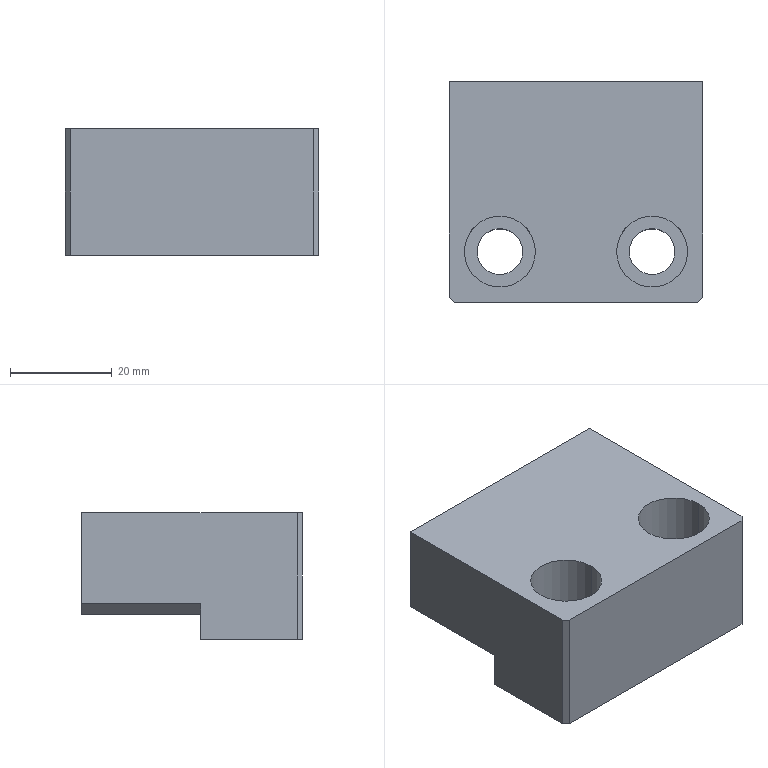Part | STEP file | J454-EBZ05-28-00-Part-1 | 1 solid | 36 faces | box 50 x 43.5 x 25 mm | volume 41584 mm3 | cylinder 16 | plane 16 | cone 4 | commonest cylinder face diameters 6.9 x4 8 x4 9 x4 14 x4
STEP:
#1=CARTESIAN_POINT('',(-15.,13.427,5.));
#2=VERTEX_POINT('',#1);
#3=CARTESIAN_POINT('',(-15.,15.5,8.45));
#4=VERTEX_POINT('',#3);
#5=CARTESIAN_POINT('',(-15.,15.5,8.45));
#6=DIRECTION('',(0.,0.515,0.8572));
#7=VECTOR('',#6,1000.);
#8=LINE('',#5,#7);
#9=EDGE_CURVE('',#2,#4,#8,.T.);
#10=ORIENTED_EDGE('',*,*,#9,.F.);
#11=CARTESIAN_POINT('',(-15.,15.5,1.55));
#12=VERTEX_POINT('',#11);
#13=CARTESIAN_POINT('',(-15.,15.5,1.55));
#14=DIRECTION('',(0.,0.515,-0.8572));
#15=VECTOR('',#14,1000.);
#16=LINE('',#13,#15);
#17=EDGE_CURVE('',#2,#12,#16,.T.);
#18=ORIENTED_EDGE('',*,*,#17,.T.);
#19=CARTESIAN_POINT('',(-15.,15.5,5.));
#20=DIRECTION('',(0.,1.,0.));
#21=DIRECTION('',(0.,0.,1.));
#22=AXIS2_PLACEMENT_3D('',#19,#20,#21);
#23=CIRCLE('',#22,3.45);
#24=EDGE_CURVE('',#12,#4,#23,.T.);
#25=ORIENTED_EDGE('',*,*,#24,.T.);
#26=EDGE_LOOP('',(#10,#18,#25));
#27=FACE_OUTER_BOUND('',#26,.T.);
#28=CARTESIAN_POINT('',(-15.,15.5,5.));
#29=DIRECTION('',(0.,1.,0.));
#30=DIRECTION('',(0.,0.,1.));
#31=AXIS2_PLACEMENT_3D('',#28,#29,#30);
#32=CONICAL_SURFACE('',#31,3.45,1.03);
#33=ADVANCED_FACE('',(#27),#32,.F.);
#34=ORIENTED_EDGE('',*,*,#24,.F.);
#35=CARTESIAN_POINT('',(-15.,17.5,1.55));
#36=VERTEX_POINT('',#35);
#37=CARTESIAN_POINT('',(-15.,33.5,1.55));
#38=DIRECTION('',(0.,1.,0.));
#39=VECTOR('',#38,1000.);
#40=LINE('',#37,#39);
#41=EDGE_CURVE('',#12,#36,#40,.T.);
#42=ORIENTED_EDGE('',*,*,#41,.T.);
#43=CARTESIAN_POINT('',(-15.,17.5,8.45));
#44=VERTEX_POINT('',#43);
#45=CARTESIAN_POINT('',(-15.,17.5,5.));
#46=DIRECTION('',(0.,1.,0.));
#47=DIRECTION('',(0.,0.,1.));
#48=AXIS2_PLACEMENT_3D('',#45,#46,#47);
#49=CIRCLE('',#48,3.45);
#50=EDGE_CURVE('',#36,#44,#49,.T.);
#51=ORIENTED_EDGE('',*,*,#50,.T.);
#52=CARTESIAN_POINT('',(-15.,33.5,8.45));
#53=DIRECTION('',(0.,1.,0.));
#54=VECTOR('',#53,1000.);
#55=LINE('',#52,#54);
#56=EDGE_CURVE('',#4,#44,#55,.T.);
#57=ORIENTED_EDGE('',*,*,#56,.F.);
#58=EDGE_LOOP('',(#34,#42,#51,#57));
#59=FACE_OUTER_BOUND('',#58,.T.);
#60=CARTESIAN_POINT('',(-15.,33.5,5.));
#61=DIRECTION('',(0.,1.,0.));
#62=DIRECTION('',(0.,0.,1.));
#63=AXIS2_PLACEMENT_3D('',#60,#61,#62);
#64=CYLINDRICAL_SURFACE('',#63,3.45);
#65=ADVANCED_FACE('',(#59),#64,.F.);
#66=CARTESIAN_POINT('',(-15.,17.5,1.));
#67=VERTEX_POINT('',#66);
#68=CARTESIAN_POINT('',(-15.,17.5,9.));
#69=VERTEX_POINT('',#68);
#70=CARTESIAN_POINT('',(-15.,17.5,5.));
#71=DIRECTION('',(0.,1.,0.));
#72=DIRECTION('',(0.,0.,1.));
#73=AXIS2_PLACEMENT_3D('',#70,#71,#72);
#74=CIRCLE('',#73,4.);
#75=EDGE_CURVE('',#67,#69,#74,.T.);
#76=ORIENTED_EDGE('',*,*,#75,.F.);
#77=CARTESIAN_POINT('',(-15.,33.5,1.));
#78=VERTEX_POINT('',#77);
#79=CARTESIAN_POINT('',(-15.,33.5,1.));
#80=DIRECTION('',(0.,1.,0.));
#81=VECTOR('',#80,1000.);
#82=LINE('',#79,#81);
#83=EDGE_CURVE('',#67,#78,#82,.T.);
#84=ORIENTED_EDGE('',*,*,#83,.T.);
#85=CARTESIAN_POINT('',(-15.,33.5,9.));
#86=VERTEX_POINT('',#85);
#87=CARTESIAN_POINT('',(-15.,33.5,5.));
#88=DIRECTION('',(0.,1.,0.));
#89=DIRECTION('',(0.,0.,1.));
#90=AXIS2_PLACEMENT_3D('',#87,#88,#89);
#91=CIRCLE('',#90,4.);
#92=EDGE_CURVE('',#78,#86,#91,.T.);
#93=ORIENTED_EDGE('',*,*,#92,.T.);
#94=CARTESIAN_POINT('',(-15.,33.5,9.));
#95=DIRECTION('',(0.,1.,0.));
#96=VECTOR('',#95,1000.);
#97=LINE('',#94,#96);
#98=EDGE_CURVE('',#69,#86,#97,.T.);
#99=ORIENTED_EDGE('',*,*,#98,.F.);
#100=EDGE_LOOP('',(#76,#84,#93,#99));
#101=FACE_OUTER_BOUND('',#100,.T.);
#102=CARTESIAN_POINT('',(-15.,33.5,5.));
#103=DIRECTION('',(0.,1.,0.));
#104=DIRECTION('',(0.,0.,1.));
#105=AXIS2_PLACEMENT_3D('',#102,#103,#104);
#106=CYLINDRICAL_SURFACE('',#105,4.);
#107=ADVANCED_FACE('',(#101),#106,.F.);
#108=CARTESIAN_POINT('',(15.,13.427,5.));
#109=VERTEX_POINT('',#108);
#110=CARTESIAN_POINT('',(15.,15.5,8.45));
#111=VERTEX_POINT('',#110);
#112=CARTESIAN_POINT('',(15.,15.5,8.45));
#113=DIRECTION('',(0.,0.515,0.8572));
#114=VECTOR('',#113,1000.);
#115=LINE('',#112,#114);
#116=EDGE_CURVE('',#109,#111,#115,.T.);
#117=ORIENTED_EDGE('',*,*,#116,.F.);
#118=CARTESIAN_POINT('',(15.,15.5,1.55));
#119=VERTEX_POINT('',#118);
#120=CARTESIAN_POINT('',(15.,15.5,1.55));
#121=DIRECTION('',(0.,0.515,-0.8572));
#122=VECTOR('',#121,1000.);
#123=LINE('',#120,#122);
#124=EDGE_CURVE('',#109,#119,#123,.T.);
#125=ORIENTED_EDGE('',*,*,#124,.T.);
#126=CARTESIAN_POINT('',(15.,15.5,5.));
#127=DIRECTION('',(0.,1.,0.));
#128=DIRECTION('',(0.,0.,1.));
#129=AXIS2_PLACEMENT_3D('',#126,#127,#128);
#130=CIRCLE('',#129,3.45);
#131=EDGE_CURVE('',#119,#111,#130,.T.);
#132=ORIENTED_EDGE('',*,*,#131,.T.);
#133=EDGE_LOOP('',(#117,#125,#132));
#134=FACE_OUTER_BOUND('',#133,.T.);
#135=CARTESIAN_POINT('',(15.,15.5,5.));
#136=DIRECTION('',(0.,1.,0.));
#137=DIRECTION('',(0.,0.,1.));
#138=AXIS2_PLACEMENT_3D('',#135,#136,#137);
#139=CONICAL_SURFACE('',#138,3.45,1.03);
#140=ADVANCED_FACE('',(#134),#139,.F.);
#141=ORIENTED_EDGE('',*,*,#131,.F.);
#142=CARTESIAN_POINT('',(15.,17.5,1.55));
#143=VERTEX_POINT('',#142);
#144=CARTESIAN_POINT('',(15.,33.5,1.55));
#145=DIRECTION('',(0.,1.,0.));
#146=VECTOR('',#145,1000.);
#147=LINE('',#144,#146);
#148=EDGE_CURVE('',#119,#143,#147,.T.);
#149=ORIENTED_EDGE('',*,*,#148,.T.);
#150=CARTESIAN_POINT('',(15.,17.5,8.45));
#151=VERTEX_POINT('',#150);
#152=CARTESIAN_POINT('',(15.,17.5,5.));
#153=DIRECTION('',(0.,1.,0.));
#154=DIRECTION('',(0.,0.,1.));
#155=AXIS2_PLACEMENT_3D('',#152,#153,#154);
#156=CIRCLE('',#155,3.45);
#157=EDGE_CURVE('',#143,#151,#156,.T.);
#158=ORIENTED_EDGE('',*,*,#157,.T.);
#159=CARTESIAN_POINT('',(15.,33.5,8.45));
#160=DIRECTION('',(0.,1.,0.));
#161=VECTOR('',#160,1000.);
#162=LINE('',#159,#161);
#163=EDGE_CURVE('',#111,#151,#162,.T.);
#164=ORIENTED_EDGE('',*,*,#163,.F.);
#165=EDGE_LOOP('',(#141,#149,#158,#164));
#166=FACE_OUTER_BOUND('',#165,.T.);
#167=CARTESIAN_POINT('',(15.,33.5,5.));
#168=DIRECTION('',(0.,1.,0.));
#169=DIRECTION('',(0.,0.,1.));
#170=AXIS2_PLACEMENT_3D('',#167,#168,#169);
#171=CYLINDRICAL_SURFACE('',#170,3.45);
#172=ADVANCED_FACE('',(#166),#171,.F.);
#173=CARTESIAN_POINT('',(15.,17.5,1.));
#174=VERTEX_POINT('',#173);
#175=CARTESIAN_POINT('',(15.,17.5,9.));
#176=VERTEX_POINT('',#175);
#177=CARTESIAN_POINT('',(15.,17.5,5.));
#178=DIRECTION('',(0.,1.,0.));
#179=DIRECTION('',(0.,0.,1.));
#180=AXIS2_PLACEMENT_3D('',#177,#178,#179);
#181=CIRCLE('',#180,4.);
#182=EDGE_CURVE('',#174,#176,#181,.T.);
#183=ORIENTED_EDGE('',*,*,#182,.F.);
#184=CARTESIAN_POINT('',(15.,33.5,1.));
#185=VERTEX_POINT('',#184);
#186=CARTESIAN_POINT('',(15.,33.5,1.));
#187=DIRECTION('',(0.,1.,0.));
#188=VECTOR('',#187,1000.);
#189=LINE('',#186,#188);
#190=EDGE_CURVE('',#174,#185,#189,.T.);
#191=ORIENTED_EDGE('',*,*,#190,.T.);
#192=CARTESIAN_POINT('',(15.,33.5,9.));
#193=VERTEX_POINT('',#192);
#194=CARTESIAN_POINT('',(15.,33.5,5.));
#195=DIRECTION('',(0.,1.,0.));
#196=DIRECTION('',(0.,0.,1.));
#197=AXIS2_PLACEMENT_3D('',#194,#195,#196);
#198=CIRCLE('',#197,4.);
#199=EDGE_CURVE('',#185,#193,#198,.T.);
#200=ORIENTED_EDGE('',*,*,#199,.T.);
#201=CARTESIAN_POINT('',(15.,33.5,9.));
#202=DIRECTION('',(0.,1.,0.));
#203=VECTOR('',#202,1000.);
#204=LINE('',#201,#203);
#205=EDGE_CURVE('',#176,#193,#204,.T.);
#206=ORIENTED_EDGE('',*,*,#205,.F.);
#207=EDGE_LOOP('',(#183,#191,#200,#206));
#208=FACE_OUTER_BOUND('',#207,.T.);
#209=CARTESIAN_POINT('',(15.,33.5,5.));
#210=DIRECTION('',(0.,1.,0.));
#211=DIRECTION('',(0.,0.,1.));
#212=AXIS2_PLACEMENT_3D('',#209,#210,#211);
#213=CYLINDRICAL_SURFACE('',#212,4.);
#214=ADVANCED_FACE('',(#208),#213,.F.);
#215=CARTESIAN_POINT('',(19.5,0.,-10.));
#216=VERTEX_POINT('',#215);
#217=CARTESIAN_POINT('',(10.5,0.,-10.));
#218=VERTEX_POINT('',#217);
#219=CARTESIAN_POINT('',(15.,0.,-10.));
#220=DIRECTION('',(0.,0.,1.));
#221=DIRECTION('',(-1.,0.,0.));
#222=AXIS2_PLACEMENT_3D('',#219,#220,#221);
#223=CIRCLE('',#222,4.5);
#224=EDGE_CURVE('',#216,#218,#223,.T.);
#225=ORIENTED_EDGE('',*,*,#224,.F.);
#226=CARTESIAN_POINT('',(19.5,0.,5.));
#227=VERTEX_POINT('',#226);
#228=CARTESIAN_POINT('',(19.5,0.,15.));
#229=DIRECTION('',(0.,0.,1.));
#230=VECTOR('',#229,1000.);
#231=LINE('',#228,#230);
#232=EDGE_CURVE('',#216,#227,#231,.T.);
#233=ORIENTED_EDGE('',*,*,#232,.T.);
#234=CARTESIAN_POINT('',(10.5,0.,5.));
#235=VERTEX_POINT('',#234);
#236=CARTESIAN_POINT('',(15.,0.,5.));
#237=DIRECTION('',(0.,0.,1.));
#238=DIRECTION('',(-1.,0.,0.));
#239=AXIS2_PLACEMENT_3D('',#236,#237,#238);
#240=CIRCLE('',#239,4.5);
#241=EDGE_CURVE('',#227,#235,#240,.T.);
#242=ORIENTED_EDGE('',*,*,#241,.T.);
#243=CARTESIAN_POINT('',(10.5,0.,15.));
#244=DIRECTION('',(0.,0.,1.));
#245=VECTOR('',#244,1000.);
#246=LINE('',#243,#245);
#247=EDGE_CURVE('',#218,#235,#246,.T.);
#248=ORIENTED_EDGE('',*,*,#247,.F.);
#249=EDGE_LOOP('',(#225,#233,#242,#248));
#250=FACE_OUTER_BOUND('',#249,.T.);
#251=CARTESIAN_POINT('',(15.,0.,15.));
#252=DIRECTION('',(0.,0.,1.));
#253=DIRECTION('',(-1.,0.,0.));
#254=AXIS2_PLACEMENT_3D('',#251,#252,#253);
#255=CYLINDRICAL_SURFACE('',#254,4.5);
#256=ADVANCED_FACE('',(#250),#255,.F.);
#257=CARTESIAN_POINT('',(22.,0.,5.));
#258=VERTEX_POINT('',#257);
#259=CARTESIAN_POINT('',(8.,0.,5.));
#260=VERTEX_POINT('',#259);
#261=CARTESIAN_POINT('',(15.,0.,5.));
#262=DIRECTION('',(0.,0.,1.));
#263=DIRECTION('',(-1.,0.,0.));
#264=AXIS2_PLACEMENT_3D('',#261,#262,#263);
#265=CIRCLE('',#264,7.);
#266=EDGE_CURVE('',#258,#260,#265,.T.);
#267=ORIENTED_EDGE('',*,*,#266,.F.);
#268=CARTESIAN_POINT('',(22.,0.,15.));
#269=VERTEX_POINT('',#268);
#270=CARTESIAN_POINT('',(22.,0.,15.));
#271=DIRECTION('',(0.,0.,1.));
#272=VECTOR('',#271,1000.);
#273=LINE('',#270,#272);
#274=EDGE_CURVE('',#258,#269,#273,.T.);
#275=ORIENTED_EDGE('',*,*,#274,.T.);
#276=CARTESIAN_POINT('',(8.,0.,15.));
#277=VERTEX_POINT('',#276);
#278=CARTESIAN_POINT('',(15.,0.,15.));
#279=DIRECTION('',(0.,0.,1.));
#280=DIRECTION('',(-1.,0.,0.));
#281=AXIS2_PLACEMENT_3D('',#278,#279,#280);
#282=CIRCLE('',#281,7.);
#283=EDGE_CURVE('',#269,#277,#282,.T.);
#284=ORIENTED_EDGE('',*,*,#283,.T.);
#285=CARTESIAN_POINT('',(8.,0.,15.));
#286=DIRECTION('',(0.,0.,1.));
#287=VECTOR('',#286,1000.);
#288=LINE('',#285,#287);
#289=EDGE_CURVE('',#260,#277,#288,.T.);
#290=ORIENTED_EDGE('',*,*,#289,.F.);
#291=EDGE_LOOP('',(#267,#275,#284,#290));
#292=FACE_OUTER_BOUND('',#291,.T.);
#293=CARTESIAN_POINT('',(15.,0.,15.));
#294=DIRECTION('',(0.,0.,1.));
#295=DIRECTION('',(-1.,0.,0.));
#296=AXIS2_PLACEMENT_3D('',#293,#294,#295);
#297=CYLINDRICAL_SURFACE('',#296,7.);
#298=ADVANCED_FACE('',(#292),#297,.F.);
#299=CARTESIAN_POINT('',(-10.5,0.,-10.));
#300=VERTEX_POINT('',#299);
#301=CARTESIAN_POINT('',(-19.5,0.,-10.));
#302=VERTEX_POINT('',#301);
#303=CARTESIAN_POINT('',(-15.,0.,-10.));
#304=DIRECTION('',(0.,0.,1.));
#305=DIRECTION('',(-1.,0.,0.));
#306=AXIS2_PLACEMENT_3D('',#303,#304,#305);
#307=CIRCLE('',#306,4.5);
#308=EDGE_CURVE('',#300,#302,#307,.T.);
#309=ORIENTED_EDGE('',*,*,#308,.F.);
#310=CARTESIAN_POINT('',(-10.5,0.,5.));
#311=VERTEX_POINT('',#310);
#312=CARTESIAN_POINT('',(-10.5,0.,15.));
#313=DIRECTION('',(0.,0.,1.));
#314=VECTOR('',#313,1000.);
#315=LINE('',#312,#314);
#316=EDGE_CURVE('',#300,#311,#315,.T.);
#317=ORIENTED_EDGE('',*,*,#316,.T.);
#318=CARTESIAN_POINT('',(-19.5,0.,5.));
#319=VERTEX_POINT('',#318);
#320=CARTESIAN_POINT('',(-15.,0.,5.));
#321=DIRECTION('',(0.,0.,1.));
#322=DIRECTION('',(-1.,0.,0.));
#323=AXIS2_PLACEMENT_3D('',#320,#321,#322);
#324=CIRCLE('',#323,4.5);
#325=EDGE_CURVE('',#311,#319,#324,.T.);
#326=ORIENTED_EDGE('',*,*,#325,.T.);
#327=CARTESIAN_POINT('',(-19.5,0.,15.));
#328=DIRECTION('',(0.,0.,1.));
#329=VECTOR('',#328,1000.);
#330=LINE('',#327,#329);
#331=EDGE_CURVE('',#302,#319,#330,.T.);
#332=ORIENTED_EDGE('',*,*,#331,.F.);
#333=EDGE_LOOP('',(#309,#317,#326,#332));
#334=FACE_OUTER_BOUND('',#333,.T.);
#335=CARTESIAN_POINT('',(-15.,0.,15.));
#336=DIRECTION('',(0.,0.,1.));
#337=DIRECTION('',(-1.,0.,0.));
#338=AXIS2_PLACEMENT_3D('',#335,#336,#337);
#339=CYLINDRICAL_SURFACE('',#338,4.5);
#340=ADVANCED_FACE('',(#334),#339,.F.);
#341=CARTESIAN_POINT('',(-8.,0.,5.));
#342=VERTEX_POINT('',#341);
#343=CARTESIAN_POINT('',(-22.,0.,5.));
#344=VERTEX_POINT('',#343);
#345=CARTESIAN_POINT('',(-15.,0.,5.));
#346=DIRECTION('',(0.,0.,1.));
#347=DIRECTION('',(-1.,0.,0.));
#348=AXIS2_PLACEMENT_3D('',#345,#346,#347);
#349=CIRCLE('',#348,7.);
#350=EDGE_CURVE('',#342,#344,#349,.T.);
#351=ORIENTED_EDGE('',*,*,#350,.F.);
#352=CARTESIAN_POINT('',(-8.,0.,15.));
#353=VERTEX_POINT('',#352);
#354=CARTESIAN_POINT('',(-8.,0.,15.));
#355=DIRECTION('',(0.,0.,1.));
#356=VECTOR('',#355,1000.);
#357=LINE('',#354,#356);
#358=EDGE_CURVE('',#342,#353,#357,.T.);
#359=ORIENTED_EDGE('',*,*,#358,.T.);
#360=CARTESIAN_POINT('',(-22.,0.,15.));
#361=VERTEX_POINT('',#360);
#362=CARTESIAN_POINT('',(-15.,0.,15.));
#363=DIRECTION('',(0.,0.,1.));
#364=DIRECTION('',(-1.,0.,0.));
#365=AXIS2_PLACEMENT_3D('',#362,#363,#364);
#366=CIRCLE('',#365,7.);
#367=EDGE_CURVE('',#353,#361,#366,.T.);
#368=ORIENTED_EDGE('',*,*,#367,.T.);
#369=CARTESIAN_POINT('',(-22.,0.,15.));
#370=DIRECTION('',(0.,0.,1.));
#371=VECTOR('',#370,1000.);
#372=LINE('',#369,#371);
#373=EDGE_CURVE('',#344,#361,#372,.T.);
#374=ORIENTED_EDGE('',*,*,#373,.F.);
#375=EDGE_LOOP('',(#351,#359,#368,#374));
#376=FACE_OUTER_BOUND('',#375,.T.);
#377=CARTESIAN_POINT('',(-15.,0.,15.));
#378=DIRECTION('',(0.,0.,1.));
#379=DIRECTION('',(-1.,0.,0.));
#380=AXIS2_PLACEMENT_3D('',#377,#378,#379);
#381=CYLINDRICAL_SURFACE('',#380,7.);
#382=ADVANCED_FACE('',(#376),#381,.F.);
#383=CARTESIAN_POINT('',(25.,10.,-10.));
#384=VERTEX_POINT('',#383);
#385=CARTESIAN_POINT('',(25.,10.,-3.));
#386=VERTEX_POINT('',#385);
#387=CARTESIAN_POINT('',(25.,10.,-10.));
#388=DIRECTION('',(0.,0.,1.));
#389=VECTOR('',#388,1000.);
#390=LINE('',#387,#389);
#391=EDGE_CURVE('',#384,#386,#390,.T.);
#392=ORIENTED_EDGE('',*,*,#391,.T.);
#393=CARTESIAN_POINT('',(25.,33.5,-3.));
#394=VERTEX_POINT('',#393);
#395=CARTESIAN_POINT('',(25.,21.905,-3.));
#396=DIRECTION('',(0.,1.,0.));
#397=VECTOR('',#396,1000.);
#398=LINE('',#395,#397);
#399=EDGE_CURVE('',#386,#394,#398,.T.);
#400=ORIENTED_EDGE('',*,*,#399,.T.);
#401=CARTESIAN_POINT('',(25.,33.5,15.));
#402=VERTEX_POINT('',#401);
#403=CARTESIAN_POINT('',(25.,33.5,-20.405));
#404=DIRECTION('',(0.,0.,-1.));
#405=VECTOR('',#404,1000.);
#406=LINE('',#403,#405);
#407=EDGE_CURVE('',#402,#394,#406,.T.);
#408=ORIENTED_EDGE('',*,*,#407,.F.);
#409=CARTESIAN_POINT('',(25.,-9.,15.));
#410=VERTEX_POINT('',#409);
#411=CARTESIAN_POINT('',(25.,-9.,15.));
#412=DIRECTION('',(0.,1.,0.));
#413=VECTOR('',#412,1000.);
#414=LINE('',#411,#413);
#415=EDGE_CURVE('',#410,#402,#414,.T.);
#416=ORIENTED_EDGE('',*,*,#415,.F.);
#417=CARTESIAN_POINT('',(25.,-9.,-10.));
#418=VERTEX_POINT('',#417);
#419=CARTESIAN_POINT('',(25.,-9.,13.));
#420=DIRECTION('',(0.,0.,-1.));
#421=VECTOR('',#420,1000.);
#422=LINE('',#419,#421);
#423=EDGE_CURVE('',#410,#418,#422,.T.);
#424=ORIENTED_EDGE('',*,*,#423,.T.);
#425=CARTESIAN_POINT('',(25.,9.,-10.));
#426=DIRECTION('',(0.,-1.,0.));
#427=VECTOR('',#426,1000.);
#428=LINE('',#425,#427);
#429=EDGE_CURVE('',#384,#418,#428,.T.);
#430=ORIENTED_EDGE('',*,*,#429,.F.);
#431=EDGE_LOOP('',(#392,#400,#408,#416,#424,#430));
#432=FACE_OUTER_BOUND('',#431,.T.);
#433=CARTESIAN_POINT('',(25.,21.905,-20.405));
#434=DIRECTION('',(-1.,0.,0.));
#435=DIRECTION('',(0.,-1.,0.));
#436=AXIS2_PLACEMENT_3D('',#433,#434,#435);
#437=PLANE('',#436);
#438=ADVANCED_FACE('',(#432),#437,.F.);
#439=CARTESIAN_POINT('',(15.,0.,-10.));
#440=DIRECTION('',(0.,0.,1.));
#441=DIRECTION('',(-1.,0.,0.));
#442=AXIS2_PLACEMENT_3D('',#439,#440,#441);
#443=CIRCLE('',#442,4.5);
#444=EDGE_CURVE('',#218,#216,#443,.T.);
#445=ORIENTED_EDGE('',*,*,#444,.T.);
#446=ORIENTED_EDGE('',*,*,#224,.T.);
#447=EDGE_LOOP('',(#445,#446));
#448=FACE_BOUND('',#447,.T.);
#449=CARTESIAN_POINT('',(-15.,0.,-10.));
#450=DIRECTION('',(0.,0.,1.));
#451=DIRECTION('',(-1.,0.,0.));
#452=AXIS2_PLACEMENT_3D('',#449,#450,#451);
#453=CIRCLE('',#452,4.5);
#454=EDGE_CURVE('',#302,#300,#453,.T.);
#455=ORIENTED_EDGE('',*,*,#454,.T.);
#456=ORIENTED_EDGE('',*,*,#308,.T.);
#457=EDGE_LOOP('',(#455,#456));
#458=FACE_BOUND('',#457,.T.);
#459=CARTESIAN_POINT('',(-25.,10.,-10.));
#460=VERTEX_POINT('',#459);
#461=CARTESIAN_POINT('',(-25.,-9.,-10.));
#462=VERTEX_POINT('',#461);
#463=CARTESIAN_POINT('',(-25.,9.,-10.));
#464=DIRECTION('',(0.,-1.,0.));
#465=VECTOR('',#464,1000.);
#466=LINE('',#463,#465);
#467=EDGE_CURVE('',#460,#462,#466,.T.);
#468=ORIENTED_EDGE('',*,*,#467,.F.);
#469=CARTESIAN_POINT('',(0.,10.,-10.));
#470=DIRECTION('',(1.,0.,0.));
#471=VECTOR('',#470,1000.);
#472=LINE('',#469,#471);
#473=EDGE_CURVE('',#460,#384,#472,.T.);
#474=ORIENTED_EDGE('',*,*,#473,.T.);
#475=ORIENTED_EDGE('',*,*,#429,.T.);
#476=CARTESIAN_POINT('',(24.,-10.,-10.));
#477=VERTEX_POINT('',#476);
#478=CARTESIAN_POINT('',(25.,-9.,-10.));
#479=DIRECTION('',(-0.7071,-0.7071,0.));
#480=VECTOR('',#479,1000.);
#481=LINE('',#478,#480);
#482=EDGE_CURVE('',#418,#477,#481,.T.);
#483=ORIENTED_EDGE('',*,*,#482,.T.);
#484=CARTESIAN_POINT('',(-24.,-10.,-10.));
#485=VERTEX_POINT('',#484);
#486=CARTESIAN_POINT('',(24.,-10.,-10.));
#487=DIRECTION('',(-1.,0.,0.));
#488=VECTOR('',#487,1000.);
#489=LINE('',#486,#488);
#490=EDGE_CURVE('',#477,#485,#489,.T.);
#491=ORIENTED_EDGE('',*,*,#490,.T.);
#492=CARTESIAN_POINT('',(-24.,-10.,-10.));
#493=DIRECTION('',(-0.7071,0.7071,0.));
#494=VECTOR('',#493,1000.);
#495=LINE('',#492,#494);
#496=EDGE_CURVE('',#485,#462,#495,.T.);
#497=ORIENTED_EDGE('',*,*,#496,.T.);
#498=EDGE_LOOP('',(#468,#474,#475,#483,#491,#497));
#499=FACE_OUTER_BOUND('',#498,.T.);
#500=CARTESIAN_POINT('',(40.389,40.389,-10.));
#501=DIRECTION('',(0.,0.,-1.));
#502=DIRECTION('',(0.,-1.,0.));
#503=AXIS2_PLACEMENT_3D('',#500,#501,#502);
#504=PLANE('',#503);
#505=ADVANCED_FACE('',(#448,#458,#499),#504,.T.);
#506=ORIENTED_EDGE('',*,*,#423,.F.);
#507=CARTESIAN_POINT('',(24.,-10.,15.));
#508=VERTEX_POINT('',#507);
#509=CARTESIAN_POINT('',(24.,-10.,15.));
#510=DIRECTION('',(0.7071,0.7071,0.));
#511=VECTOR('',#510,1000.);
#512=LINE('',#509,#511);
#513=EDGE_CURVE('',#508,#410,#512,.T.);
#514=ORIENTED_EDGE('',*,*,#513,.F.);
#515=CARTESIAN_POINT('',(24.,-10.,13.));
#516=DIRECTION('',(0.,0.,-1.));
#517=VECTOR('',#516,1000.);
#518=LINE('',#515,#517);
#519=EDGE_CURVE('',#508,#477,#518,.T.);
#520=ORIENTED_EDGE('',*,*,#519,.T.);
#521=ORIENTED_EDGE('',*,*,#482,.F.);
#522=EDGE_LOOP('',(#506,#514,#520,#521));
#523=FACE_OUTER_BOUND('',#522,.T.);
#524=CARTESIAN_POINT('',(36.721,2.721,18.783));
#525=DIRECTION('',(0.7071,-0.7071,0.));
#526=DIRECTION('',(-0.7071,-0.7071,0.));
#527=AXIS2_PLACEMENT_3D('',#524,#525,#526);
#528=PLANE('',#527);
#529=ADVANCED_FACE('',(#523),#528,.T.);
#530=CARTESIAN_POINT('',(15.,0.,15.));
#531=DIRECTION('',(0.,0.,1.));
#532=DIRECTION('',(-1.,0.,0.));
#533=AXIS2_PLACEMENT_3D('',#530,#531,#532);
#534=CIRCLE('',#533,7.);
#535=EDGE_CURVE('',#277,#269,#534,.T.);
#536=ORIENTED_EDGE('',*,*,#535,.F.);
#537=ORIENTED_EDGE('',*,*,#283,.F.);
#538=EDGE_LOOP('',(#536,#537));
#539=FACE_BOUND('',#538,.T.);
#540=CARTESIAN_POINT('',(-15.,0.,15.));
#541=DIRECTION('',(0.,0.,1.));
#542=DIRECTION('',(-1.,0.,0.));
#543=AXIS2_PLACEMENT_3D('',#540,#541,#542);
#544=CIRCLE('',#543,7.);
#545=EDGE_CURVE('',#361,#353,#544,.T.);
#546=ORIENTED_EDGE('',*,*,#545,.F.);
#547=ORIENTED_EDGE('',*,*,#367,.F.);
#548=EDGE_LOOP('',(#546,#547));
#549=FACE_BOUND('',#548,.T.);
#550=CARTESIAN_POINT('',(-25.,-9.,15.));
#551=VERTEX_POINT('',#550);
#552=CARTESIAN_POINT('',(-25.,33.5,15.));
#553=VERTEX_POINT('',#552);
#554=CARTESIAN_POINT('',(-25.,-9.,15.));
#555=DIRECTION('',(0.,1.,0.));
#556=VECTOR('',#555,1000.);
#557=LINE('',#554,#556);
#558=EDGE_CURVE('',#551,#553,#557,.T.);
#559=ORIENTED_EDGE('',*,*,#558,.F.);
#560=CARTESIAN_POINT('',(-24.,-10.,15.));
#561=VERTEX_POINT('',#560);
#562=CARTESIAN_POINT('',(-25.,-9.,15.));
#563=DIRECTION('',(0.7071,-0.7071,0.));
#564=VECTOR('',#563,1000.);
#565=LINE('',#562,#564);
#566=EDGE_CURVE('',#551,#561,#565,.T.);
#567=ORIENTED_EDGE('',*,*,#566,.T.);
#568=CARTESIAN_POINT('',(24.,-10.,15.));
#569=DIRECTION('',(-1.,0.,0.));
#570=VECTOR('',#569,1000.);
#571=LINE('',#568,#570);
#572=EDGE_CURVE('',#508,#561,#571,.T.);
#573=ORIENTED_EDGE('',*,*,#572,.F.);
#574=ORIENTED_EDGE('',*,*,#513,.T.);
#575=ORIENTED_EDGE('',*,*,#415,.T.);
#576=CARTESIAN_POINT('',(24.,33.5,15.));
#577=DIRECTION('',(-1.,0.,0.));
#578=VECTOR('',#577,1000.);
#579=LINE('',#576,#578);
#580=EDGE_CURVE('',#402,#553,#579,.T.);
#581=ORIENTED_EDGE('',*,*,#580,.T.);
#582=EDGE_LOOP('',(#559,#567,#573,#574,#575,#581));
#583=FACE_OUTER_BOUND('',#582,.T.);
#584=CARTESIAN_POINT('',(40.389,-40.389,15.));
#585=DIRECTION('',(0.,0.,1.));
#586=DIRECTION('',(0.,1.,0.));
#587=AXIS2_PLACEMENT_3D('',#584,#585,#586);
#588=PLANE('',#587);
#589=ADVANCED_FACE('',(#539,#549,#583),#588,.T.);
#590=CARTESIAN_POINT('',(-15.,33.5,5.));
#591=DIRECTION('',(0.,1.,0.));
#592=DIRECTION('',(0.,0.,1.));
#593=AXIS2_PLACEMENT_3D('',#590,#591,#592);
#594=CIRCLE('',#593,4.);
#595=EDGE_CURVE('',#86,#78,#594,.T.);
#596=ORIENTED_EDGE('',*,*,#595,.F.);
#597=ORIENTED_EDGE('',*,*,#92,.F.);
#598=EDGE_LOOP('',(#596,#597));
#599=FACE_BOUND('',#598,.T.);
#600=CARTESIAN_POINT('',(15.,33.5,5.));
#601=DIRECTION('',(0.,1.,0.));
#602=DIRECTION('',(0.,0.,1.));
#603=AXIS2_PLACEMENT_3D('',#600,#601,#602);
#604=CIRCLE('',#603,4.);
#605=EDGE_CURVE('',#193,#185,#604,.T.);
#606=ORIENTED_EDGE('',*,*,#605,.F.);
#607=ORIENTED_EDGE('',*,*,#199,.F.);
#608=EDGE_LOOP('',(#606,#607));
#609=FACE_BOUND('',#608,.T.);
#610=ORIENTED_EDGE('',*,*,#407,.T.);
#611=CARTESIAN_POINT('',(23.,33.5,-5.));
#612=VERTEX_POINT('',#611);
#613=CARTESIAN_POINT('',(54.669,33.5,26.669));
#614=DIRECTION('',(-0.7071,0.,-0.7071));
#615=VECTOR('',#614,1000.);
#616=LINE('',#613,#615);
#617=EDGE_CURVE('',#394,#612,#616,.T.);
#618=ORIENTED_EDGE('',*,*,#617,.T.);
#619=CARTESIAN_POINT('',(-23.,33.5,-5.));
#620=VERTEX_POINT('',#619);
#621=CARTESIAN_POINT('',(39.919,33.5,-5.));
#622=DIRECTION('',(1.,0.,0.));
#623=VECTOR('',#622,1000.);
#624=LINE('',#621,#623);
#625=EDGE_CURVE('',#620,#612,#624,.T.);
#626=ORIENTED_EDGE('',*,*,#625,.F.);
#627=CARTESIAN_POINT('',(-25.,33.5,-3.));
#628=VERTEX_POINT('',#627);
#629=CARTESIAN_POINT('',(-14.75,33.5,-13.25));
#630=DIRECTION('',(-0.7071,0.,0.7071));
#631=VECTOR('',#630,1000.);
#632=LINE('',#629,#631);
#633=EDGE_CURVE('',#620,#628,#632,.T.);
#634=ORIENTED_EDGE('',*,*,#633,.T.);
#635=CARTESIAN_POINT('',(-25.,33.5,-20.405));
#636=DIRECTION('',(0.,0.,1.));
#637=VECTOR('',#636,1000.);
#638=LINE('',#635,#637);
#639=EDGE_CURVE('',#628,#553,#638,.T.);
#640=ORIENTED_EDGE('',*,*,#639,.T.);
#641=ORIENTED_EDGE('',*,*,#580,.F.);
#642=EDGE_LOOP('',(#610,#618,#626,#634,#640,#641));
#643=FACE_OUTER_BOUND('',#642,.T.);
#644=CARTESIAN_POINT('',(39.919,33.5,41.419));
#645=DIRECTION('',(0.,1.,0.));
#646=DIRECTION('',(0.,0.,-1.));
#647=AXIS2_PLACEMENT_3D('',#644,#645,#646);
#648=PLANE('',#647);
#649=ADVANCED_FACE('',(#599,#609,#643),#648,.T.);
#650=ORIENTED_EDGE('',*,*,#490,.F.);
#651=ORIENTED_EDGE('',*,*,#519,.F.);
#652=ORIENTED_EDGE('',*,*,#572,.T.);
#653=CARTESIAN_POINT('',(-24.,-10.,-10.));
#654=DIRECTION('',(0.,0.,1.));
#655=VECTOR('',#654,1000.);
#656=LINE('',#653,#655);
#657=EDGE_CURVE('',#485,#561,#656,.T.);
#658=ORIENTED_EDGE('',*,*,#657,.F.);
#659=EDGE_LOOP('',(#650,#651,#652,#658));
#660=FACE_OUTER_BOUND('',#659,.T.);
#661=CARTESIAN_POINT('',(39.919,-10.,-38.419));
#662=DIRECTION('',(0.,-1.,0.));
#663=DIRECTION('',(0.,0.,1.));
#664=AXIS2_PLACEMENT_3D('',#661,#662,#663);
#665=PLANE('',#664);
#666=ADVANCED_FACE('',(#660),#665,.T.);
#667=CARTESIAN_POINT('',(-25.,-9.,-10.));
#668=DIRECTION('',(0.,0.,1.));
#669=VECTOR('',#668,1000.);
#670=LINE('',#667,#669);
#671=EDGE_CURVE('',#462,#551,#670,.T.);
#672=ORIENTED_EDGE('',*,*,#671,.F.);
#673=ORIENTED_EDGE('',*,*,#496,.F.);
#674=ORIENTED_EDGE('',*,*,#657,.T.);
#675=ORIENTED_EDGE('',*,*,#566,.F.);
#676=EDGE_LOOP('',(#672,#673,#674,#675));
#677=FACE_OUTER_BOUND('',#676,.T.);
#678=CARTESIAN_POINT('',(-36.721,2.721,-15.783));
#679=DIRECTION('',(-0.7071,-0.7071,0.));
#680=DIRECTION('',(0.7071,-0.7071,0.));
#681=AXIS2_PLACEMENT_3D('',#678,#679,#680);
#682=PLANE('',#681);
#683=ADVANCED_FACE('',(#677),#682,.T.);
#684=ORIENTED_EDGE('',*,*,#639,.F.);
#685=CARTESIAN_POINT('',(-25.,10.,-3.));
#686=VERTEX_POINT('',#685);
#687=CARTESIAN_POINT('',(-25.,10.,-3.));
#688=DIRECTION('',(0.,-1.,0.));
#689=VECTOR('',#688,1000.);
#690=LINE('',#687,#689);
#691=EDGE_CURVE('',#628,#686,#690,.T.);
#692=ORIENTED_EDGE('',*,*,#691,.T.);
#693=CARTESIAN_POINT('',(-25.,10.,-10.));
#694=DIRECTION('',(0.,0.,1.));
#695=VECTOR('',#694,1000.);
#696=LINE('',#693,#695);
#697=EDGE_CURVE('',#460,#686,#696,.T.);
#698=ORIENTED_EDGE('',*,*,#697,.F.);
#699=ORIENTED_EDGE('',*,*,#467,.T.);
#700=ORIENTED_EDGE('',*,*,#671,.T.);
#701=ORIENTED_EDGE('',*,*,#558,.T.);
#702=EDGE_LOOP('',(#684,#692,#698,#699,#700,#701));
#703=FACE_OUTER_BOUND('',#702,.T.);
#704=CARTESIAN_POINT('',(-25.,21.905,-20.405));
#705=DIRECTION('',(-1.,0.,0.));
#706=DIRECTION('',(0.,-1.,0.));
#707=AXIS2_PLACEMENT_3D('',#704,#705,#706);
#708=PLANE('',#707);
#709=ADVANCED_FACE('',(#703),#708,.T.);
#710=ORIENTED_EDGE('',*,*,#358,.F.);
#711=CARTESIAN_POINT('',(-15.,0.,5.));
#712=DIRECTION('',(0.,0.,1.));
#713=DIRECTION('',(-1.,0.,0.));
#714=AXIS2_PLACEMENT_3D('',#711,#712,#713);
#715=CIRCLE('',#714,7.);
#716=EDGE_CURVE('',#344,#342,#715,.T.);
#717=ORIENTED_EDGE('',*,*,#716,.F.);
#718=ORIENTED_EDGE('',*,*,#373,.T.);
#719=ORIENTED_EDGE('',*,*,#545,.T.);
#720=EDGE_LOOP('',(#710,#717,#718,#719));
#721=FACE_OUTER_BOUND('',#720,.T.);
#722=CARTESIAN_POINT('',(-15.,0.,15.));
#723=DIRECTION('',(0.,0.,1.));
#724=DIRECTION('',(-1.,0.,0.));
#725=AXIS2_PLACEMENT_3D('',#722,#723,#724);
#726=CYLINDRICAL_SURFACE('',#725,7.);
#727=ADVANCED_FACE('',(#721),#726,.F.);
#728=CARTESIAN_POINT('',(-15.,0.,5.));
#729=DIRECTION('',(0.,0.,1.));
#730=DIRECTION('',(-1.,0.,0.));
#731=AXIS2_PLACEMENT_3D('',#728,#729,#730);
#732=CIRCLE('',#731,4.5);
#733=EDGE_CURVE('',#319,#311,#732,.T.);
#734=ORIENTED_EDGE('',*,*,#733,.F.);
#735=ORIENTED_EDGE('',*,*,#325,.F.);
#736=EDGE_LOOP('',(#734,#735));
#737=FACE_BOUND('',#736,.T.);
#738=ORIENTED_EDGE('',*,*,#716,.T.);
#739=ORIENTED_EDGE('',*,*,#350,.T.);
#740=EDGE_LOOP('',(#738,#739));
#741=FACE_OUTER_BOUND('',#740,.T.);
#742=CARTESIAN_POINT('',(-8.,0.,5.));
#743=DIRECTION('',(0.,0.,-1.));
#744=DIRECTION('',(1.,0.,0.));
#745=AXIS2_PLACEMENT_3D('',#742,#743,#744);
#746=PLANE('',#745);
#747=ADVANCED_FACE('',(#737,#741),#746,.F.);
#748=ORIENTED_EDGE('',*,*,#316,.F.);
#749=ORIENTED_EDGE('',*,*,#454,.F.);
#750=ORIENTED_EDGE('',*,*,#331,.T.);
#751=ORIENTED_EDGE('',*,*,#733,.T.);
#752=EDGE_LOOP('',(#748,#749,#750,#751));
#753=FACE_OUTER_BOUND('',#752,.T.);
#754=CARTESIAN_POINT('',(-15.,0.,15.));
#755=DIRECTION('',(0.,0.,1.));
#756=DIRECTION('',(-1.,0.,0.));
#757=AXIS2_PLACEMENT_3D('',#754,#755,#756);
#758=CYLINDRICAL_SURFACE('',#757,4.5);
#759=ADVANCED_FACE('',(#753),#758,.F.);
#760=ORIENTED_EDGE('',*,*,#274,.F.);
#761=CARTESIAN_POINT('',(15.,0.,5.));
#762=DIRECTION('',(0.,0.,1.));
#763=DIRECTION('',(-1.,0.,0.));
#764=AXIS2_PLACEMENT_3D('',#761,#762,#763);
#765=CIRCLE('',#764,7.);
#766=EDGE_CURVE('',#260,#258,#765,.T.);
#767=ORIENTED_EDGE('',*,*,#766,.F.);
#768=ORIENTED_EDGE('',*,*,#289,.T.);
#769=ORIENTED_EDGE('',*,*,#535,.T.);
#770=EDGE_LOOP('',(#760,#767,#768,#769));
#771=FACE_OUTER_BOUND('',#770,.T.);
#772=CARTESIAN_POINT('',(15.,0.,15.));
#773=DIRECTION('',(0.,0.,1.));
#774=DIRECTION('',(-1.,0.,0.));
#775=AXIS2_PLACEMENT_3D('',#772,#773,#774);
#776=CYLINDRICAL_SURFACE('',#775,7.);
#777=ADVANCED_FACE('',(#771),#776,.F.);
#778=CARTESIAN_POINT('',(15.,0.,5.));
#779=DIRECTION('',(0.,0.,1.));
#780=DIRECTION('',(-1.,0.,0.));
#781=AXIS2_PLACEMENT_3D('',#778,#779,#780);
#782=CIRCLE('',#781,4.5);
#783=EDGE_CURVE('',#235,#227,#782,.T.);
#784=ORIENTED_EDGE('',*,*,#783,.F.);
#785=ORIENTED_EDGE('',*,*,#241,.F.);
#786=EDGE_LOOP('',(#784,#785));
#787=FACE_BOUND('',#786,.T.);
#788=ORIENTED_EDGE('',*,*,#766,.T.);
#789=ORIENTED_EDGE('',*,*,#266,.T.);
#790=EDGE_LOOP('',(#788,#789));
#791=FACE_OUTER_BOUND('',#790,.T.);
#792=CARTESIAN_POINT('',(22.,0.,5.));
#793=DIRECTION('',(0.,0.,-1.));
#794=DIRECTION('',(1.,0.,0.));
#795=AXIS2_PLACEMENT_3D('',#792,#793,#794);
#796=PLANE('',#795);
#797=ADVANCED_FACE('',(#787,#791),#796,.F.);
#798=ORIENTED_EDGE('',*,*,#232,.F.);
#799=ORIENTED_EDGE('',*,*,#444,.F.);
#800=ORIENTED_EDGE('',*,*,#247,.T.);
#801=ORIENTED_EDGE('',*,*,#783,.T.);
#802=EDGE_LOOP('',(#798,#799,#800,#801));
#803=FACE_OUTER_BOUND('',#802,.T.);
#804=CARTESIAN_POINT('',(15.,0.,15.));
#805=DIRECTION('',(0.,0.,1.));
#806=DIRECTION('',(-1.,0.,0.));
#807=AXIS2_PLACEMENT_3D('',#804,#805,#806);
#808=CYLINDRICAL_SURFACE('',#807,4.5);
#809=ADVANCED_FACE('',(#803),#808,.F.);
#810=ORIENTED_EDGE('',*,*,#625,.T.);
#811=CARTESIAN_POINT('',(23.,10.,-5.));
#812=VERTEX_POINT('',#811);
#813=CARTESIAN_POINT('',(23.,22.75,-5.));
#814=DIRECTION('',(0.,-1.,0.));
#815=VECTOR('',#814,1000.);
#816=LINE('',#813,#815);
#817=EDGE_CURVE('',#612,#812,#816,.T.);
#818=ORIENTED_EDGE('',*,*,#817,.T.);
#819=CARTESIAN_POINT('',(-23.,10.,-5.));
#820=VERTEX_POINT('',#819);
#821=CARTESIAN_POINT('',(0.,10.,-5.));
#822=DIRECTION('',(-1.,0.,0.));
#823=VECTOR('',#822,1000.);
#824=LINE('',#821,#823);
#825=EDGE_CURVE('',#812,#820,#824,.T.);
#826=ORIENTED_EDGE('',*,*,#825,.T.);
#827=CARTESIAN_POINT('',(-23.,33.5,-5.));
#828=DIRECTION('',(0.,1.,0.));
#829=VECTOR('',#828,1000.);
#830=LINE('',#827,#829);
#831=EDGE_CURVE('',#820,#620,#830,.T.);
#832=ORIENTED_EDGE('',*,*,#831,.T.);
#833=EDGE_LOOP('',(#810,#818,#826,#832));
#834=FACE_OUTER_BOUND('',#833,.T.);
#835=CARTESIAN_POINT('',(0.,22.75,-5.));
#836=DIRECTION('',(0.,0.,1.));
#837=DIRECTION('',(1.,0.,0.));
#838=AXIS2_PLACEMENT_3D('',#835,#836,#837);
#839=PLANE('',#838);
#840=ADVANCED_FACE('',(#834),#839,.F.);
#841=ORIENTED_EDGE('',*,*,#391,.F.);
#842=ORIENTED_EDGE('',*,*,#473,.F.);
#843=ORIENTED_EDGE('',*,*,#697,.T.);
#844=CARTESIAN_POINT('',(-9.,10.,-19.));
#845=DIRECTION('',(0.7071,0.,-0.7071));
#846=VECTOR('',#845,1000.);
#847=LINE('',#844,#846);
#848=EDGE_CURVE('',#686,#820,#847,.T.);
#849=ORIENTED_EDGE('',*,*,#848,.T.);
#850=ORIENTED_EDGE('',*,*,#825,.F.);
#851=CARTESIAN_POINT('',(9.,10.,-19.));
#852=DIRECTION('',(0.7071,0.,0.7071));
#853=VECTOR('',#852,1000.);
#854=LINE('',#851,#853);
#855=EDGE_CURVE('',#812,#386,#854,.T.);
#856=ORIENTED_EDGE('',*,*,#855,.T.);
#857=EDGE_LOOP('',(#841,#842,#843,#849,#850,#856));
#858=FACE_OUTER_BOUND('',#857,.T.);
#859=CARTESIAN_POINT('',(0.,10.,-10.));
#860=DIRECTION('',(0.,-1.,0.));
#861=DIRECTION('',(0.,0.,-1.));
#862=AXIS2_PLACEMENT_3D('',#859,#860,#861);
#863=PLANE('',#862);
#864=ADVANCED_FACE('',(#858),#863,.F.);
#865=ORIENTED_EDGE('',*,*,#848,.F.);
#866=ORIENTED_EDGE('',*,*,#691,.F.);
#867=ORIENTED_EDGE('',*,*,#633,.F.);
#868=ORIENTED_EDGE('',*,*,#831,.F.);
#869=EDGE_LOOP('',(#865,#866,#867,#868));
#870=FACE_OUTER_BOUND('',#869,.T.);
#871=CARTESIAN_POINT('',(-23.,22.75,-5.));
#872=DIRECTION('',(-0.7071,0.,-0.7071));
#873=DIRECTION('',(0.,-1.,0.));
#874=AXIS2_PLACEMENT_3D('',#871,#872,#873);
#875=PLANE('',#874);
#876=ADVANCED_FACE('',(#870),#875,.T.);
#877=ORIENTED_EDGE('',*,*,#617,.F.);
#878=ORIENTED_EDGE('',*,*,#399,.F.);
#879=ORIENTED_EDGE('',*,*,#855,.F.);
#880=ORIENTED_EDGE('',*,*,#817,.F.);
#881=EDGE_LOOP('',(#877,#878,#879,#880));
#882=FACE_OUTER_BOUND('',#881,.T.);
#883=CARTESIAN_POINT('',(23.,22.75,-5.));
#884=DIRECTION('',(-0.7071,0.,0.7071));
#885=DIRECTION('',(0.,-1.,0.));
#886=AXIS2_PLACEMENT_3D('',#883,#884,#885);
#887=PLANE('',#886);
#888=ADVANCED_FACE('',(#882),#887,.F.);
#889=ORIENTED_EDGE('',*,*,#190,.F.);
#890=CARTESIAN_POINT('',(15.,17.5,5.));
#891=DIRECTION('',(0.,1.,0.));
#892=DIRECTION('',(0.,0.,1.));
#893=AXIS2_PLACEMENT_3D('',#890,#891,#892);
#894=CIRCLE('',#893,4.);
#895=EDGE_CURVE('',#176,#174,#894,.T.);
#896=ORIENTED_EDGE('',*,*,#895,.F.);
#897=ORIENTED_EDGE('',*,*,#205,.T.);
#898=ORIENTED_EDGE('',*,*,#605,.T.);
#899=EDGE_LOOP('',(#889,#896,#897,#898));
#900=FACE_OUTER_BOUND('',#899,.T.);
#901=CARTESIAN_POINT('',(15.,33.5,5.));
#902=DIRECTION('',(0.,1.,0.));
#903=DIRECTION('',(0.,0.,1.));
#904=AXIS2_PLACEMENT_3D('',#901,#902,#903);
#905=CYLINDRICAL_SURFACE('',#904,4.);
#906=ADVANCED_FACE('',(#900),#905,.F.);
#907=CARTESIAN_POINT('',(15.,17.5,5.));
#908=DIRECTION('',(0.,1.,0.));
#909=DIRECTION('',(0.,0.,1.));
#910=AXIS2_PLACEMENT_3D('',#907,#908,#909);
#911=CIRCLE('',#910,3.45);
#912=EDGE_CURVE('',#151,#143,#911,.T.);
#913=ORIENTED_EDGE('',*,*,#912,.F.);
#914=ORIENTED_EDGE('',*,*,#157,.F.);
#915=EDGE_LOOP('',(#913,#914));
#916=FACE_BOUND('',#915,.T.);
#917=ORIENTED_EDGE('',*,*,#895,.T.);
#918=ORIENTED_EDGE('',*,*,#182,.T.);
#919=EDGE_LOOP('',(#917,#918));
#920=FACE_OUTER_BOUND('',#919,.T.);
#921=CARTESIAN_POINT('',(15.,17.5,1.));
#922=DIRECTION('',(0.,-1.,0.));
#923=DIRECTION('',(0.,0.,-1.));
#924=AXIS2_PLACEMENT_3D('',#921,#922,#923);
#925=PLANE('',#924);
#926=ADVANCED_FACE('',(#916,#920),#925,.F.);
#927=ORIENTED_EDGE('',*,*,#148,.F.);
#928=CARTESIAN_POINT('',(15.,15.5,5.));
#929=DIRECTION('',(0.,1.,0.));
#930=DIRECTION('',(0.,0.,1.));
#931=AXIS2_PLACEMENT_3D('',#928,#929,#930);
#932=CIRCLE('',#931,3.45);
#933=EDGE_CURVE('',#111,#119,#932,.T.);
#934=ORIENTED_EDGE('',*,*,#933,.F.);
#935=ORIENTED_EDGE('',*,*,#163,.T.);
#936=ORIENTED_EDGE('',*,*,#912,.T.);
#937=EDGE_LOOP('',(#927,#934,#935,#936));
#938=FACE_OUTER_BOUND('',#937,.T.);
#939=CARTESIAN_POINT('',(15.,33.5,5.));
#940=DIRECTION('',(0.,1.,0.));
#941=DIRECTION('',(0.,0.,1.));
#942=AXIS2_PLACEMENT_3D('',#939,#940,#941);
#943=CYLINDRICAL_SURFACE('',#942,3.45);
#944=ADVANCED_FACE('',(#938),#943,.F.);
#945=ORIENTED_EDGE('',*,*,#124,.F.);
#946=ORIENTED_EDGE('',*,*,#116,.T.);
#947=ORIENTED_EDGE('',*,*,#933,.T.);
#948=EDGE_LOOP('',(#945,#946,#947));
#949=FACE_OUTER_BOUND('',#948,.T.);
#950=CARTESIAN_POINT('',(15.,15.5,5.));
#951=DIRECTION('',(0.,1.,0.));
#952=DIRECTION('',(0.,0.,1.));
#953=AXIS2_PLACEMENT_3D('',#950,#951,#952);
#954=CONICAL_SURFACE('',#953,3.45,1.03);
#955=ADVANCED_FACE('',(#949),#954,.F.);
#956=ORIENTED_EDGE('',*,*,#83,.F.);
#957=CARTESIAN_POINT('',(-15.,17.5,5.));
#958=DIRECTION('',(0.,1.,0.));
#959=DIRECTION('',(0.,0.,1.));
#960=AXIS2_PLACEMENT_3D('',#957,#958,#959);
#961=CIRCLE('',#960,4.);
#962=EDGE_CURVE('',#69,#67,#961,.T.);
#963=ORIENTED_EDGE('',*,*,#962,.F.);
#964=ORIENTED_EDGE('',*,*,#98,.T.);
#965=ORIENTED_EDGE('',*,*,#595,.T.);
#966=EDGE_LOOP('',(#956,#963,#964,#965));
#967=FACE_OUTER_BOUND('',#966,.T.);
#968=CARTESIAN_POINT('',(-15.,33.5,5.));
#969=DIRECTION('',(0.,1.,0.));
#970=DIRECTION('',(0.,0.,1.));
#971=AXIS2_PLACEMENT_3D('',#968,#969,#970);
#972=CYLINDRICAL_SURFACE('',#971,4.);
#973=ADVANCED_FACE('',(#967),#972,.F.);
#974=CARTESIAN_POINT('',(-15.,17.5,5.));
#975=DIRECTION('',(0.,1.,0.));
#976=DIRECTION('',(0.,0.,1.));
#977=AXIS2_PLACEMENT_3D('',#974,#975,#976);
#978=CIRCLE('',#977,3.45);
#979=EDGE_CURVE('',#44,#36,#978,.T.);
#980=ORIENTED_EDGE('',*,*,#979,.F.);
#981=ORIENTED_EDGE('',*,*,#50,.F.);
#982=EDGE_LOOP('',(#980,#981));
#983=FACE_BOUND('',#982,.T.);
#984=ORIENTED_EDGE('',*,*,#962,.T.);
#985=ORIENTED_EDGE('',*,*,#75,.T.);
#986=EDGE_LOOP('',(#984,#985));
#987=FACE_OUTER_BOUND('',#986,.T.);
#988=CARTESIAN_POINT('',(-15.,17.5,1.));
#989=DIRECTION('',(0.,-1.,0.));
#990=DIRECTION('',(0.,0.,-1.));
#991=AXIS2_PLACEMENT_3D('',#988,#989,#990);
#992=PLANE('',#991);
#993=ADVANCED_FACE('',(#983,#987),#992,.F.);
#994=ORIENTED_EDGE('',*,*,#41,.F.);
#995=CARTESIAN_POINT('',(-15.,15.5,5.));
#996=DIRECTION('',(0.,1.,0.));
#997=DIRECTION('',(0.,0.,1.));
#998=AXIS2_PLACEMENT_3D('',#995,#996,#997);
#999=CIRCLE('',#998,3.45);
#1000=EDGE_CURVE('',#4,#12,#999,.T.);
#1001=ORIENTED_EDGE('',*,*,#1000,.F.);
#1002=ORIENTED_EDGE('',*,*,#56,.T.);
#1003=ORIENTED_EDGE('',*,*,#979,.T.);
#1004=EDGE_LOOP('',(#994,#1001,#1002,#1003));
#1005=FACE_OUTER_BOUND('',#1004,.T.);
#1006=CARTESIAN_POINT('',(-15.,33.5,5.));
#1007=DIRECTION('',(0.,1.,0.));
#1008=DIRECTION('',(0.,0.,1.));
#1009=AXIS2_PLACEMENT_3D('',#1006,#1007,#1008);
#1010=CYLINDRICAL_SURFACE('',#1009,3.45);
#1011=ADVANCED_FACE('',(#1005),#1010,.F.);
#1012=ORIENTED_EDGE('',*,*,#17,.F.);
#1013=ORIENTED_EDGE('',*,*,#9,.T.);
#1014=ORIENTED_EDGE('',*,*,#1000,.T.);
#1015=EDGE_LOOP('',(#1012,#1013,#1014));
#1016=FACE_OUTER_BOUND('',#1015,.T.);
#1017=CARTESIAN_POINT('',(-15.,15.5,5.));
#1018=DIRECTION('',(0.,1.,0.));
#1019=DIRECTION('',(0.,0.,1.));
#1020=AXIS2_PLACEMENT_3D('',#1017,#1018,#1019);
#1021=CONICAL_SURFACE('',#1020,3.45,1.03);
#1022=ADVANCED_FACE('',(#1016),#1021,.F.);
#1023=CLOSED_SHELL('',(#33,#65,#107,#140,#172,#214,#256,#298,#340,#382,#438,#505,#529,#589,#649,#666,#683,#709,#727,#747,#759,#777,#797,#809,#840,#864,#876,#888,#906,#926,#944,#955,#973,#993,#1011,#1022));
#1024=MANIFOLD_SOLID_BREP('',#1023);
#1025=CARTESIAN_POINT('',(0.,0.,0.));
#1026=DIRECTION('',(0.,0.,1.));
#1027=DIRECTION('',(1.,0.,0.));
#1028=AXIS2_PLACEMENT_3D('',#1025,#1026,#1027);
#1029=(LENGTH_UNIT()NAMED_UNIT(*)SI_UNIT(.MILLI.,.METRE.));
#1030=UNCERTAINTY_MEASURE_WITH_UNIT(LENGTH_MEASURE(0.00001),#1029,'','');
#1031=(NAMED_UNIT(*)PLANE_ANGLE_UNIT()SI_UNIT($,.RADIAN.));
#1032=(NAMED_UNIT(*)SI_UNIT($,.STERADIAN.)SOLID_ANGLE_UNIT());
#1033=(GEOMETRIC_REPRESENTATION_CONTEXT(3)GLOBAL_UNCERTAINTY_ASSIGNED_CONTEXT((#1030))GLOBAL_UNIT_ASSIGNED_CONTEXT((#1029,#1031,#1032))REPRESENTATION_CONTEXT('',''));
#1034=ADVANCED_BREP_SHAPE_REPRESENTATION('',(#1024,#1028),#1033);